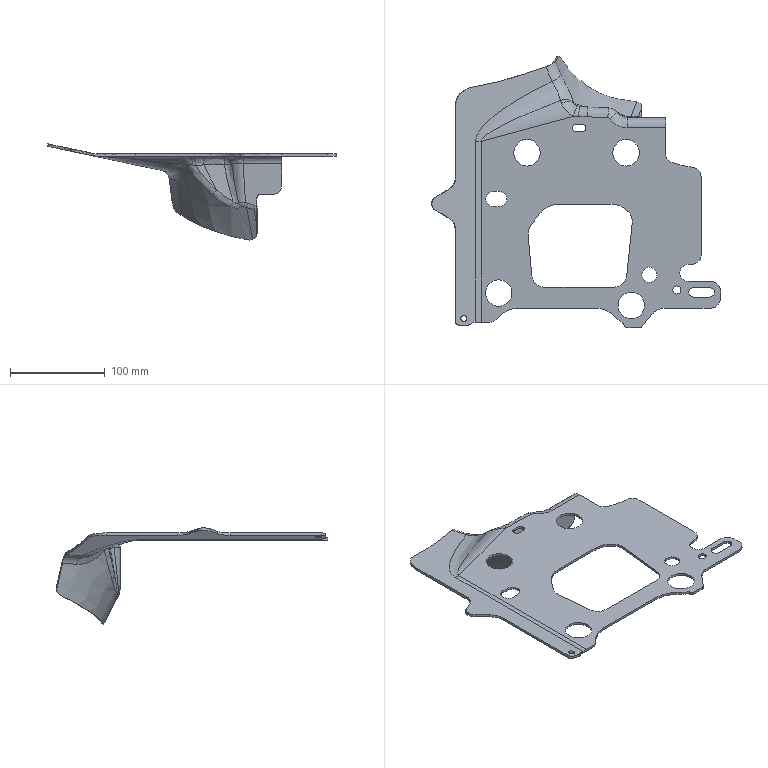Part | STEP file | K8D2-17C930-A-INS-01_id26_x_t | 1 solid | 153 faces | box 305 x 286.849 x 101.505 mm | volume 137938 mm3 | spline 83 | cylinder 44 | plane 26 | commonest cylinder face diameters 20 x6 8 x5 16 x4 28 x4 30 x3 50 x3